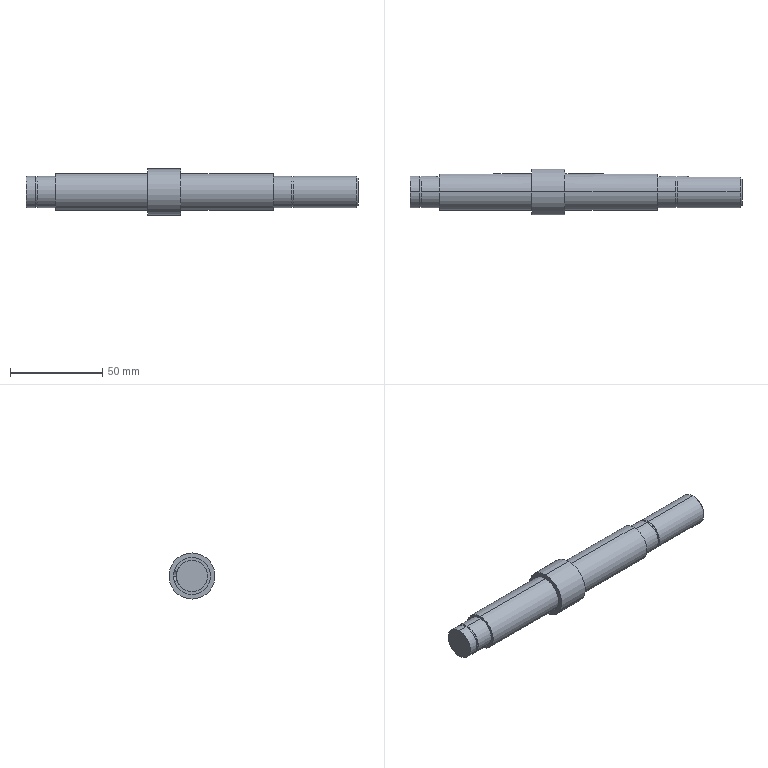Part | STEP file | CON-006 | 1 solid | 50 faces | box 180 x 25 x 25 mm | volume 52361 mm3 | cylinder 28 | plane 19 | cone 3 | commonest cylinder face diameters 6 x10 17 x8 16.2 x4 20 x4 25 x2